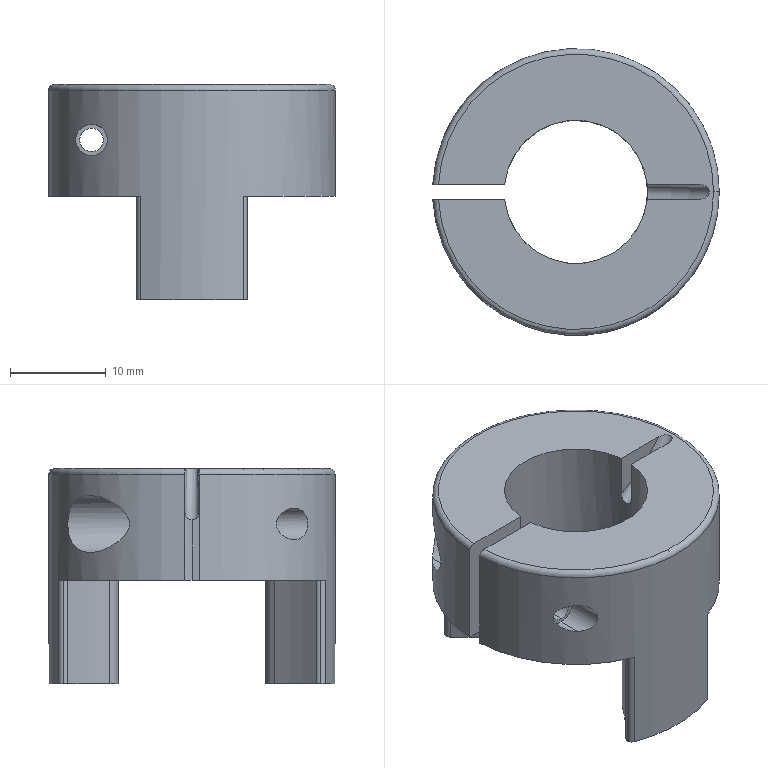Part | STEP file | BODY-R_E-LMPJC30L35-14-15-LK5 | 1 solid | 37 faces | box 29.981 x 30 x 22.5 mm | volume 6898 mm3 | cylinder 24 | plane 10 | torus 3 | commonest cylinder face diameters 1.2 x6 61.94 x4 2.459 x2 3.2 x2 3.3 x2 4.3 x2